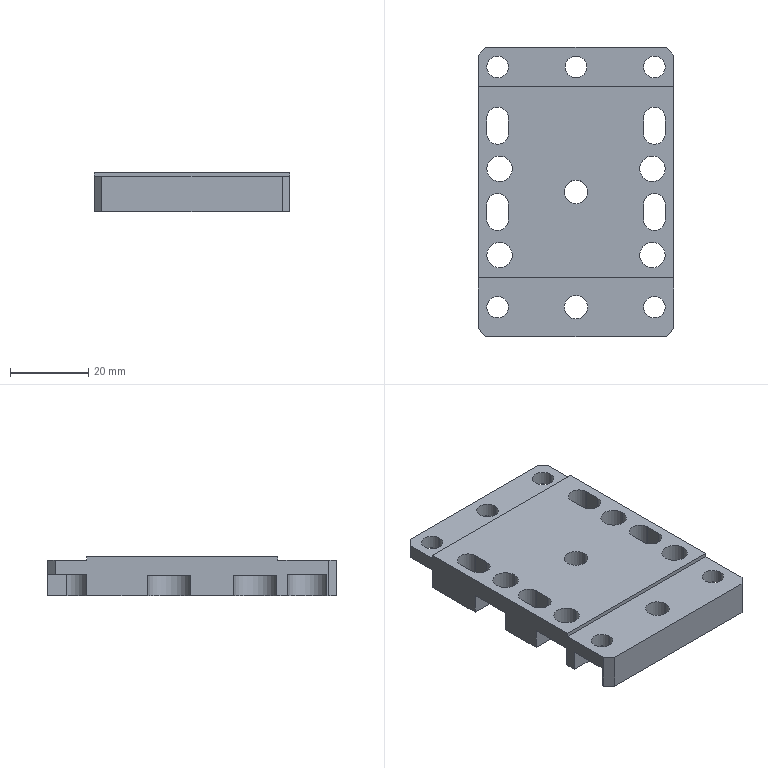Part | STEP file | 04-02-02 small base plate | 1 solid | 91 faces | box 50 x 73.8 x 10 mm | volume 27452 mm3 | plane 49 | cylinder 42 | commonest cylinder face diameters 5.5 x18 6.5 x8 10 x6 11 x6 6 x4